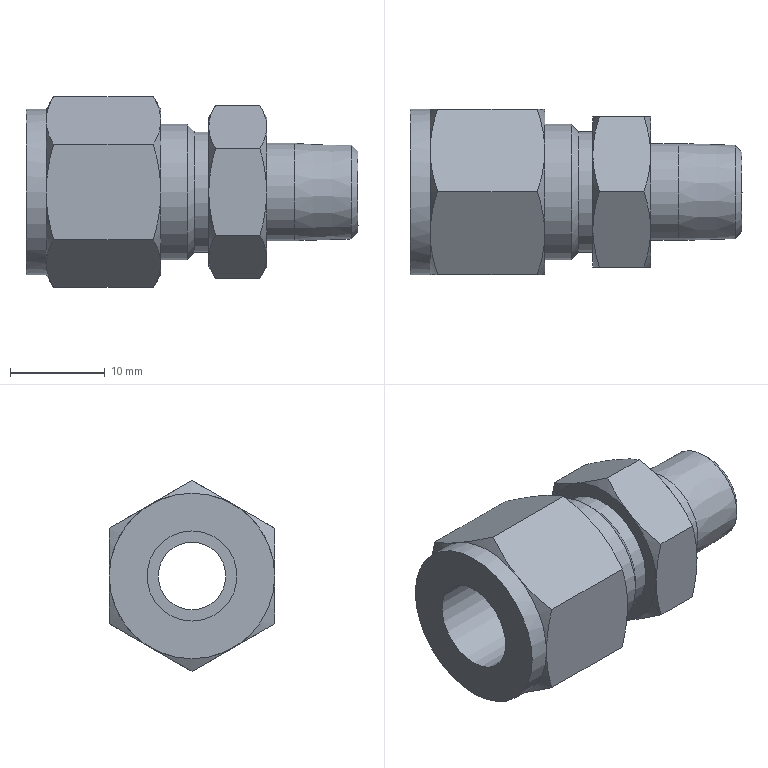Part | STEP file | LUMP1 | 1 solid | 51 faces | box 35.052 x 17.463 x 20.164 mm | volume 4534 mm3 | cone 27 | plane 18 | cylinder 6 | commonest cylinder face diameters 7.137 x1 9.525 x1 10.287 x1 12.776 x1 14.287 x1 17.462 x1